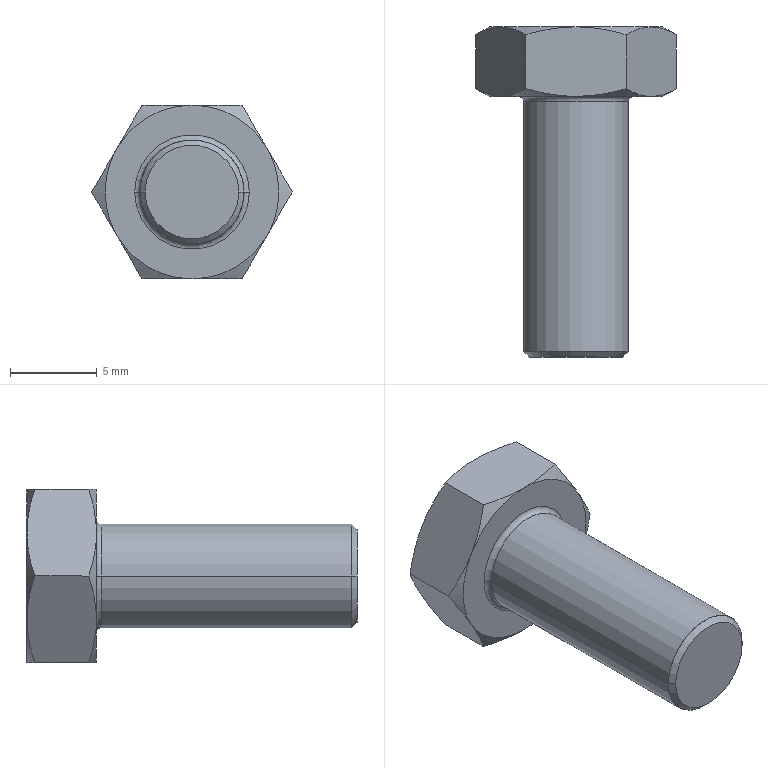Part | NX | features BREP 2 | 1 solid | 31 faces | box 11.547 x 19 x 10 mm | volume 976.022 mm3 | cone 14 | plane 11 | cylinder 4 | torus 2 | commonest cylinder face diameters 4.917 x2 6 x2